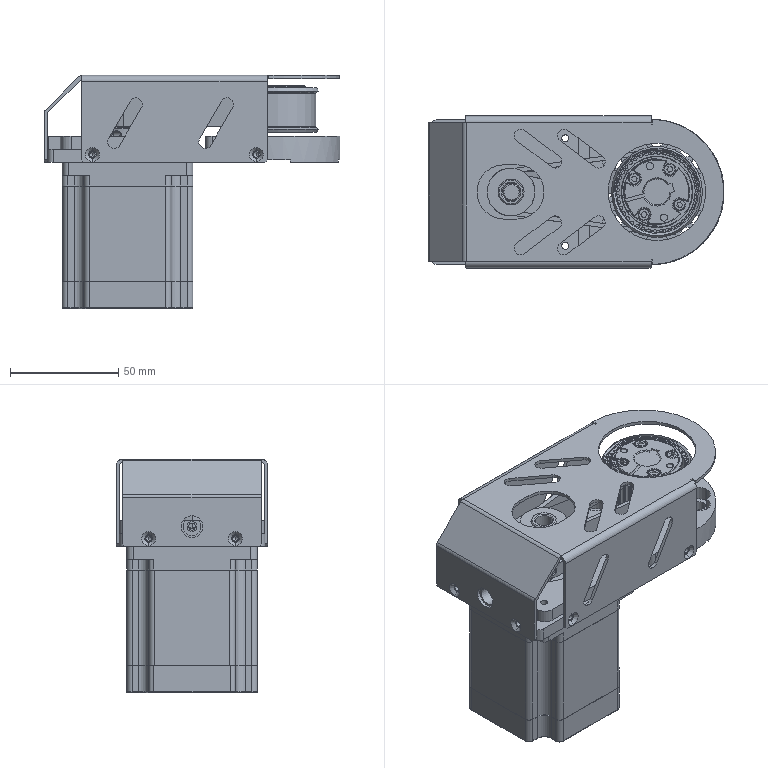Part | STEP file | Copy of C0045-60 side link 2:1(K60)^K50A-1H20-S(formula driven)-L700-motor left- | 10 solids | 985 faces | box 136.5 x 70 x 107.5 mm | volume 328495 mm3 | cylinder 570 | plane 261 | cone 118 | spline 32 | torus 4 | commonest cylinder face diameters 0.6 x160 1.82 x79 37.44 x40 6 x38 5 x24 19.1 x21